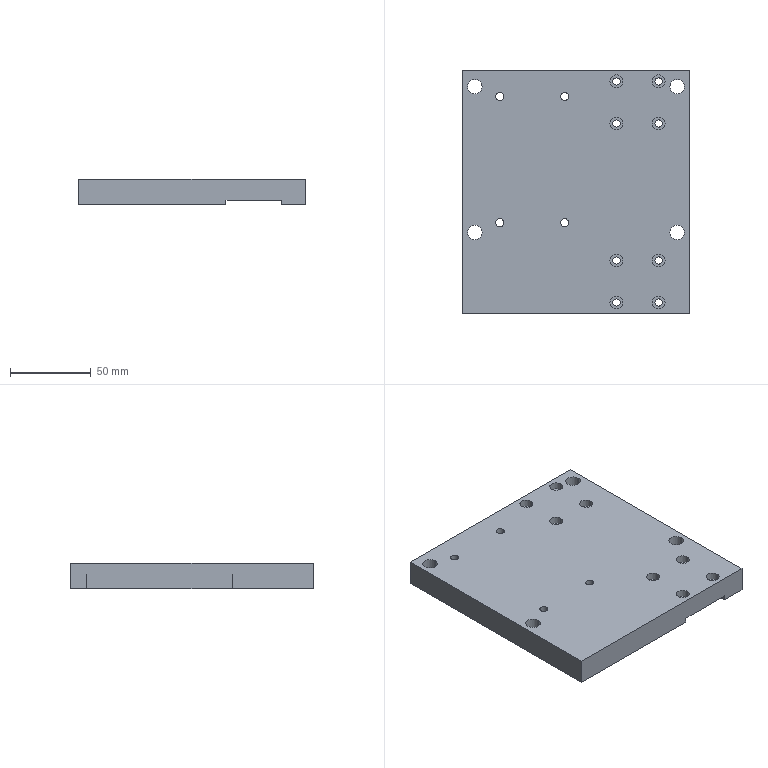Part | STEP file | X77-04003 | 1 solid | 86 faces | box 140 x 150 x 16 mm | volume 308847 mm3 | cylinder 60 | plane 22 | cone 4 | commonest cylinder face diameters 4.5 x16 8 x16 5 x8 9 x8 14 x8 4.2 x4